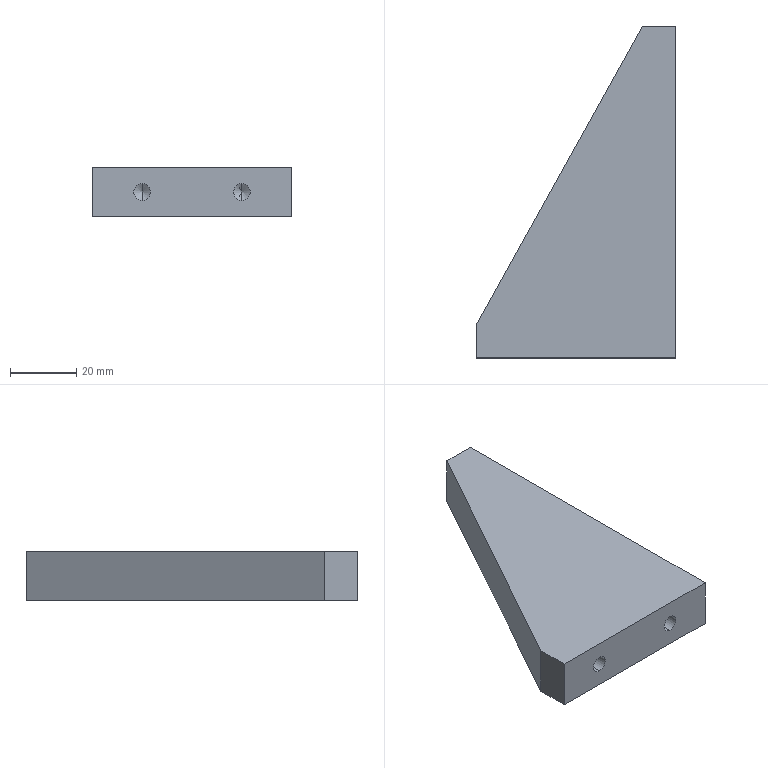Part | SolidWorks | features BaseBody 1 | 1 solid | 27 faces | box 60 x 100 x 15 mm | volume 54728 mm3 | cylinder 10 | cone 10 | plane 7 | commonest cylinder face diameters 5 x10
STEP:
#1=CARTESIAN_POINT('',(-15.,25.,2.5));
#2=VERTEX_POINT('',#1);
#3=CARTESIAN_POINT('',(-15.,25.,-2.5));
#4=VERTEX_POINT('',#3);
#5=CARTESIAN_POINT('',(-15.,25.,0.));
#6=DIRECTION('',(1.,0.,0.));
#7=DIRECTION('',(0.,0.,-1.));
#8=AXIS2_PLACEMENT_3D('',#5,#6,#7);
#9=CIRCLE('',#8,2.5);
#10=EDGE_CURVE('',#2,#4,#9,.T.);
#11=ORIENTED_EDGE('',*,*,#10,.F.);
#12=CARTESIAN_POINT('',(0.,25.,2.5));
#13=VERTEX_POINT('',#12);
#14=CARTESIAN_POINT('',(0.,25.,2.5));
#15=DIRECTION('',(1.,0.,0.));
#16=VECTOR('',#15,1000.);
#17=LINE('',#14,#16);
#18=EDGE_CURVE('',#2,#13,#17,.T.);
#19=ORIENTED_EDGE('',*,*,#18,.T.);
#20=CARTESIAN_POINT('',(0.,25.,-2.5));
#21=VERTEX_POINT('',#20);
#22=CARTESIAN_POINT('',(0.,25.,0.));
#23=DIRECTION('',(1.,0.,0.));
#24=DIRECTION('',(0.,0.,-1.));
#25=AXIS2_PLACEMENT_3D('',#22,#23,#24);
#26=CIRCLE('',#25,2.5);
#27=EDGE_CURVE('',#13,#21,#26,.T.);
#28=ORIENTED_EDGE('',*,*,#27,.T.);
#29=CARTESIAN_POINT('',(0.,25.,-2.5));
#30=DIRECTION('',(1.,0.,0.));
#31=VECTOR('',#30,1000.);
#32=LINE('',#29,#31);
#33=EDGE_CURVE('',#4,#21,#32,.T.);
#34=ORIENTED_EDGE('',*,*,#33,.F.);
#35=EDGE_LOOP('',(#11,#19,#28,#34));
#36=FACE_OUTER_BOUND('',#35,.T.);
#37=CARTESIAN_POINT('',(0.,25.,0.));
#38=DIRECTION('',(1.,0.,0.));
#39=DIRECTION('',(0.,0.,-1.));
#40=AXIS2_PLACEMENT_3D('',#37,#38,#39);
#41=CYLINDRICAL_SURFACE('',#40,2.5);
#42=ADVANCED_FACE('',(#36),#41,.F.);
#43=CARTESIAN_POINT('',(-16.502,25.,0.));
#44=VERTEX_POINT('',#43);
#45=CARTESIAN_POINT('',(-15.,25.,-2.5));
#46=DIRECTION('',(0.515,0.,-0.8572));
#47=VECTOR('',#46,1000.);
#48=LINE('',#45,#47);
#49=EDGE_CURVE('',#44,#4,#48,.T.);
#50=ORIENTED_EDGE('',*,*,#49,.F.);
#51=CARTESIAN_POINT('',(-15.,25.,2.5));
#52=DIRECTION('',(0.515,0.,0.8572));
#53=VECTOR('',#52,1000.);
#54=LINE('',#51,#53);
#55=EDGE_CURVE('',#44,#2,#54,.T.);
#56=ORIENTED_EDGE('',*,*,#55,.T.);
#57=ORIENTED_EDGE('',*,*,#10,.T.);
#58=EDGE_LOOP('',(#50,#56,#57));
#59=FACE_OUTER_BOUND('',#58,.T.);
#60=CARTESIAN_POINT('',(-15.,25.,0.));
#61=DIRECTION('',(1.,0.,0.));
#62=DIRECTION('',(0.,0.,-1.));
#63=AXIS2_PLACEMENT_3D('',#60,#61,#62);
#64=CONICAL_SURFACE('',#63,2.5,1.03);
#65=ADVANCED_FACE('',(#59),#64,.F.);
#66=CARTESIAN_POINT('',(-15.,55.,2.5));
#67=VERTEX_POINT('',#66);
#68=CARTESIAN_POINT('',(-15.,55.,-2.5));
#69=VERTEX_POINT('',#68);
#70=CARTESIAN_POINT('',(-15.,55.,0.));
#71=DIRECTION('',(1.,0.,0.));
#72=DIRECTION('',(0.,0.,-1.));
#73=AXIS2_PLACEMENT_3D('',#70,#71,#72);
#74=CIRCLE('',#73,2.5);
#75=EDGE_CURVE('',#67,#69,#74,.T.);
#76=ORIENTED_EDGE('',*,*,#75,.F.);
#77=CARTESIAN_POINT('',(0.,55.,2.5));
#78=VERTEX_POINT('',#77);
#79=CARTESIAN_POINT('',(0.,55.,2.5));
#80=DIRECTION('',(1.,0.,0.));
#81=VECTOR('',#80,1000.);
#82=LINE('',#79,#81);
#83=EDGE_CURVE('',#67,#78,#82,.T.);
#84=ORIENTED_EDGE('',*,*,#83,.T.);
#85=CARTESIAN_POINT('',(0.,55.,-2.5));
#86=VERTEX_POINT('',#85);
#87=CARTESIAN_POINT('',(0.,55.,0.));
#88=DIRECTION('',(1.,0.,0.));
#89=DIRECTION('',(0.,0.,-1.));
#90=AXIS2_PLACEMENT_3D('',#87,#88,#89);
#91=CIRCLE('',#90,2.5);
#92=EDGE_CURVE('',#78,#86,#91,.T.);
#93=ORIENTED_EDGE('',*,*,#92,.T.);
#94=CARTESIAN_POINT('',(0.,55.,-2.5));
#95=DIRECTION('',(1.,0.,0.));
#96=VECTOR('',#95,1000.);
#97=LINE('',#94,#96);
#98=EDGE_CURVE('',#69,#86,#97,.T.);
#99=ORIENTED_EDGE('',*,*,#98,.F.);
#100=EDGE_LOOP('',(#76,#84,#93,#99));
#101=FACE_OUTER_BOUND('',#100,.T.);
#102=CARTESIAN_POINT('',(0.,55.,0.));
#103=DIRECTION('',(1.,0.,0.));
#104=DIRECTION('',(0.,0.,-1.));
#105=AXIS2_PLACEMENT_3D('',#102,#103,#104);
#106=CYLINDRICAL_SURFACE('',#105,2.5);
#107=ADVANCED_FACE('',(#101),#106,.F.);
#108=CARTESIAN_POINT('',(-16.502,55.,0.));
#109=VERTEX_POINT('',#108);
#110=CARTESIAN_POINT('',(-15.,55.,-2.5));
#111=DIRECTION('',(0.515,0.,-0.8572));
#112=VECTOR('',#111,1000.);
#113=LINE('',#110,#112);
#114=EDGE_CURVE('',#109,#69,#113,.T.);
#115=ORIENTED_EDGE('',*,*,#114,.F.);
#116=CARTESIAN_POINT('',(-15.,55.,2.5));
#117=DIRECTION('',(0.515,0.,0.8572));
#118=VECTOR('',#117,1000.);
#119=LINE('',#116,#118);
#120=EDGE_CURVE('',#109,#67,#119,.T.);
#121=ORIENTED_EDGE('',*,*,#120,.T.);
#122=ORIENTED_EDGE('',*,*,#75,.T.);
#123=EDGE_LOOP('',(#115,#121,#122));
#124=FACE_OUTER_BOUND('',#123,.T.);
#125=CARTESIAN_POINT('',(-15.,55.,0.));
#126=DIRECTION('',(1.,0.,0.));
#127=DIRECTION('',(0.,0.,-1.));
#128=AXIS2_PLACEMENT_3D('',#125,#126,#127);
#129=CONICAL_SURFACE('',#128,2.5,1.03);
#130=ADVANCED_FACE('',(#124),#129,.F.);
#131=CARTESIAN_POINT('',(-15.,85.,2.5));
#132=VERTEX_POINT('',#131);
#133=CARTESIAN_POINT('',(-15.,85.,-2.5));
#134=VERTEX_POINT('',#133);
#135=CARTESIAN_POINT('',(-15.,85.,0.));
#136=DIRECTION('',(1.,0.,0.));
#137=DIRECTION('',(0.,0.,-1.));
#138=AXIS2_PLACEMENT_3D('',#135,#136,#137);
#139=CIRCLE('',#138,2.5);
#140=EDGE_CURVE('',#132,#134,#139,.T.);
#141=ORIENTED_EDGE('',*,*,#140,.F.);
#142=CARTESIAN_POINT('',(0.,85.,2.5));
#143=VERTEX_POINT('',#142);
#144=CARTESIAN_POINT('',(0.,85.,2.5));
#145=DIRECTION('',(1.,0.,0.));
#146=VECTOR('',#145,1000.);
#147=LINE('',#144,#146);
#148=EDGE_CURVE('',#132,#143,#147,.T.);
#149=ORIENTED_EDGE('',*,*,#148,.T.);
#150=CARTESIAN_POINT('',(0.,85.,-2.5));
#151=VERTEX_POINT('',#150);
#152=CARTESIAN_POINT('',(0.,85.,0.));
#153=DIRECTION('',(1.,0.,0.));
#154=DIRECTION('',(0.,0.,-1.));
#155=AXIS2_PLACEMENT_3D('',#152,#153,#154);
#156=CIRCLE('',#155,2.5);
#157=EDGE_CURVE('',#143,#151,#156,.T.);
#158=ORIENTED_EDGE('',*,*,#157,.T.);
#159=CARTESIAN_POINT('',(0.,85.,-2.5));
#160=DIRECTION('',(1.,0.,0.));
#161=VECTOR('',#160,1000.);
#162=LINE('',#159,#161);
#163=EDGE_CURVE('',#134,#151,#162,.T.);
#164=ORIENTED_EDGE('',*,*,#163,.F.);
#165=EDGE_LOOP('',(#141,#149,#158,#164));
#166=FACE_OUTER_BOUND('',#165,.T.);
#167=CARTESIAN_POINT('',(0.,85.,0.));
#168=DIRECTION('',(1.,0.,0.));
#169=DIRECTION('',(0.,0.,-1.));
#170=AXIS2_PLACEMENT_3D('',#167,#168,#169);
#171=CYLINDRICAL_SURFACE('',#170,2.5);
#172=ADVANCED_FACE('',(#166),#171,.F.);
#173=CARTESIAN_POINT('',(-16.502,85.,0.));
#174=VERTEX_POINT('',#173);
#175=CARTESIAN_POINT('',(-15.,85.,-2.5));
#176=DIRECTION('',(0.515,0.,-0.8572));
#177=VECTOR('',#176,1000.);
#178=LINE('',#175,#177);
#179=EDGE_CURVE('',#174,#134,#178,.T.);
#180=ORIENTED_EDGE('',*,*,#179,.F.);
#181=CARTESIAN_POINT('',(-15.,85.,2.5));
#182=DIRECTION('',(0.515,0.,0.8572));
#183=VECTOR('',#182,1000.);
#184=LINE('',#181,#183);
#185=EDGE_CURVE('',#174,#132,#184,.T.);
#186=ORIENTED_EDGE('',*,*,#185,.T.);
#187=ORIENTED_EDGE('',*,*,#140,.T.);
#188=EDGE_LOOP('',(#180,#186,#187));
#189=FACE_OUTER_BOUND('',#188,.T.);
#190=CARTESIAN_POINT('',(-15.,85.,0.));
#191=DIRECTION('',(1.,0.,0.));
#192=DIRECTION('',(0.,0.,-1.));
#193=AXIS2_PLACEMENT_3D('',#190,#191,#192);
#194=CONICAL_SURFACE('',#193,2.5,1.03);
#195=ADVANCED_FACE('',(#189),#194,.F.);
#196=CARTESIAN_POINT('',(-15.,15.,2.5));
#197=VERTEX_POINT('',#196);
#198=CARTESIAN_POINT('',(-15.,15.,-2.5));
#199=VERTEX_POINT('',#198);
#200=CARTESIAN_POINT('',(-15.,15.,0.));
#201=DIRECTION('',(0.,-1.,0.));
#202=DIRECTION('',(0.,0.,-1.));
#203=AXIS2_PLACEMENT_3D('',#200,#201,#202);
#204=CIRCLE('',#203,2.5);
#205=EDGE_CURVE('',#197,#199,#204,.T.);
#206=ORIENTED_EDGE('',*,*,#205,.F.);
#207=CARTESIAN_POINT('',(-15.,0.,2.5));
#208=VERTEX_POINT('',#207);
#209=CARTESIAN_POINT('',(-15.,0.,2.5));
#210=DIRECTION('',(0.,-1.,0.));
#211=VECTOR('',#210,1000.);
#212=LINE('',#209,#211);
#213=EDGE_CURVE('',#197,#208,#212,.T.);
#214=ORIENTED_EDGE('',*,*,#213,.T.);
#215=CARTESIAN_POINT('',(-15.,0.,-2.5));
#216=VERTEX_POINT('',#215);
#217=CARTESIAN_POINT('',(-15.,0.,0.));
#218=DIRECTION('',(0.,-1.,0.));
#219=DIRECTION('',(0.,0.,-1.));
#220=AXIS2_PLACEMENT_3D('',#217,#218,#219);
#221=CIRCLE('',#220,2.5);
#222=EDGE_CURVE('',#208,#216,#221,.T.);
#223=ORIENTED_EDGE('',*,*,#222,.T.);
#224=CARTESIAN_POINT('',(-15.,0.,-2.5));
#225=DIRECTION('',(0.,-1.,0.));
#226=VECTOR('',#225,1000.);
#227=LINE('',#224,#226);
#228=EDGE_CURVE('',#199,#216,#227,.T.);
#229=ORIENTED_EDGE('',*,*,#228,.F.);
#230=EDGE_LOOP('',(#206,#214,#223,#229));
#231=FACE_OUTER_BOUND('',#230,.T.);
#232=CARTESIAN_POINT('',(-15.,0.,0.));
#233=DIRECTION('',(0.,-1.,0.));
#234=DIRECTION('',(0.,0.,-1.));
#235=AXIS2_PLACEMENT_3D('',#232,#233,#234);
#236=CYLINDRICAL_SURFACE('',#235,2.5);
#237=ADVANCED_FACE('',(#231),#236,.F.);
#238=CARTESIAN_POINT('',(-15.,16.502,0.));
#239=VERTEX_POINT('',#238);
#240=CARTESIAN_POINT('',(-15.,15.,-2.5));
#241=DIRECTION('',(0.,-0.515,-0.8572));
#242=VECTOR('',#241,1000.);
#243=LINE('',#240,#242);
#244=EDGE_CURVE('',#239,#199,#243,.T.);
#245=ORIENTED_EDGE('',*,*,#244,.F.);
#246=CARTESIAN_POINT('',(-15.,15.,2.5));
#247=DIRECTION('',(0.,-0.515,0.8572));
#248=VECTOR('',#247,1000.);
#249=LINE('',#246,#248);
#250=EDGE_CURVE('',#239,#197,#249,.T.);
#251=ORIENTED_EDGE('',*,*,#250,.T.);
#252=ORIENTED_EDGE('',*,*,#205,.T.);
#253=EDGE_LOOP('',(#245,#251,#252));
#254=FACE_OUTER_BOUND('',#253,.T.);
#255=CARTESIAN_POINT('',(-15.,15.,0.));
#256=DIRECTION('',(0.,-1.,0.));
#257=DIRECTION('',(0.,0.,-1.));
#258=AXIS2_PLACEMENT_3D('',#255,#256,#257);
#259=CONICAL_SURFACE('',#258,2.5,1.03);
#260=ADVANCED_FACE('',(#254),#259,.F.);
#261=CARTESIAN_POINT('',(-45.,15.,2.5));
#262=VERTEX_POINT('',#261);
#263=CARTESIAN_POINT('',(-45.,15.,-2.5));
#264=VERTEX_POINT('',#263);
#265=CARTESIAN_POINT('',(-45.,15.,0.));
#266=DIRECTION('',(0.,-1.,0.));
#267=DIRECTION('',(0.,0.,-1.));
#268=AXIS2_PLACEMENT_3D('',#265,#266,#267);
#269=CIRCLE('',#268,2.5);
#270=EDGE_CURVE('',#262,#264,#269,.T.);
#271=ORIENTED_EDGE('',*,*,#270,.F.);
#272=CARTESIAN_POINT('',(-45.,0.,2.5));
#273=VERTEX_POINT('',#272);
#274=CARTESIAN_POINT('',(-45.,0.,2.5));
#275=DIRECTION('',(0.,-1.,0.));
#276=VECTOR('',#275,1000.);
#277=LINE('',#274,#276);
#278=EDGE_CURVE('',#262,#273,#277,.T.);
#279=ORIENTED_EDGE('',*,*,#278,.T.);
#280=CARTESIAN_POINT('',(-45.,0.,-2.5));
#281=VERTEX_POINT('',#280);
#282=CARTESIAN_POINT('',(-45.,0.,0.));
#283=DIRECTION('',(0.,-1.,0.));
#284=DIRECTION('',(0.,0.,-1.));
#285=AXIS2_PLACEMENT_3D('',#282,#283,#284);
#286=CIRCLE('',#285,2.5);
#287=EDGE_CURVE('',#273,#281,#286,.T.);
#288=ORIENTED_EDGE('',*,*,#287,.T.);
#289=CARTESIAN_POINT('',(-45.,0.,-2.5));
#290=DIRECTION('',(0.,-1.,0.));
#291=VECTOR('',#290,1000.);
#292=LINE('',#289,#291);
#293=EDGE_CURVE('',#264,#281,#292,.T.);
#294=ORIENTED_EDGE('',*,*,#293,.F.);
#295=EDGE_LOOP('',(#271,#279,#288,#294));
#296=FACE_OUTER_BOUND('',#295,.T.);
#297=CARTESIAN_POINT('',(-45.,0.,0.));
#298=DIRECTION('',(0.,-1.,0.));
#299=DIRECTION('',(0.,0.,-1.));
#300=AXIS2_PLACEMENT_3D('',#297,#298,#299);
#301=CYLINDRICAL_SURFACE('',#300,2.5);
#302=ADVANCED_FACE('',(#296),#301,.F.);
#303=CARTESIAN_POINT('',(-45.,16.502,0.));
#304=VERTEX_POINT('',#303);
#305=CARTESIAN_POINT('',(-45.,15.,-2.5));
#306=DIRECTION('',(0.,-0.515,-0.8572));
#307=VECTOR('',#306,1000.);
#308=LINE('',#305,#307);
#309=EDGE_CURVE('',#304,#264,#308,.T.);
#310=ORIENTED_EDGE('',*,*,#309,.F.);
#311=CARTESIAN_POINT('',(-45.,15.,2.5));
#312=DIRECTION('',(0.,-0.515,0.8572));
#313=VECTOR('',#312,1000.);
#314=LINE('',#311,#313);
#315=EDGE_CURVE('',#304,#262,#314,.T.);
#316=ORIENTED_EDGE('',*,*,#315,.T.);
#317=ORIENTED_EDGE('',*,*,#270,.T.);
#318=EDGE_LOOP('',(#310,#316,#317));
#319=FACE_OUTER_BOUND('',#318,.T.);
#320=CARTESIAN_POINT('',(-45.,15.,0.));
#321=DIRECTION('',(0.,-1.,0.));
#322=DIRECTION('',(0.,0.,-1.));
#323=AXIS2_PLACEMENT_3D('',#320,#321,#322);
#324=CONICAL_SURFACE('',#323,2.5,1.03);
#325=ADVANCED_FACE('',(#319),#324,.F.);
#326=CARTESIAN_POINT('',(-60.,10.,-7.5));
#327=VERTEX_POINT('',#326);
#328=CARTESIAN_POINT('',(-60.,0.,-7.5));
#329=VERTEX_POINT('',#328);
#330=CARTESIAN_POINT('',(-60.,10.,-7.5));
#331=DIRECTION('',(0.,-1.,0.));
#332=VECTOR('',#331,1000.);
#333=LINE('',#330,#332);
#334=EDGE_CURVE('',#327,#329,#333,.T.);
#335=ORIENTED_EDGE('',*,*,#334,.F.);
#336=CARTESIAN_POINT('',(-10.,100.,-7.5));
#337=VERTEX_POINT('',#336);
#338=CARTESIAN_POINT('',(-10.,100.,-7.5));
#339=DIRECTION('',(-0.4856,-0.8742,0.));
#340=VECTOR('',#339,1000.);
#341=LINE('',#338,#340);
#342=EDGE_CURVE('',#337,#327,#341,.T.);
#343=ORIENTED_EDGE('',*,*,#342,.F.);
#344=CARTESIAN_POINT('',(0.,100.,-7.5));
#345=VERTEX_POINT('',#344);
#346=CARTESIAN_POINT('',(0.,100.,-7.5));
#347=DIRECTION('',(-1.,0.,0.));
#348=VECTOR('',#347,1000.);
#349=LINE('',#346,#348);
#350=EDGE_CURVE('',#345,#337,#349,.T.);
#351=ORIENTED_EDGE('',*,*,#350,.F.);
#352=CARTESIAN_POINT('',(0.,0.,-7.5));
#353=VERTEX_POINT('',#352);
#354=CARTESIAN_POINT('',(0.,0.,-7.5));
#355=DIRECTION('',(0.,1.,0.));
#356=VECTOR('',#355,1000.);
#357=LINE('',#354,#356);
#358=EDGE_CURVE('',#353,#345,#357,.T.);
#359=ORIENTED_EDGE('',*,*,#358,.F.);
#360=CARTESIAN_POINT('',(-60.,0.,-7.5));
#361=DIRECTION('',(1.,0.,0.));
#362=VECTOR('',#361,1000.);
#363=LINE('',#360,#362);
#364=EDGE_CURVE('',#329,#353,#363,.T.);
#365=ORIENTED_EDGE('',*,*,#364,.F.);
#366=EDGE_LOOP('',(#335,#343,#351,#359,#365));
#367=FACE_OUTER_BOUND('',#366,.T.);
#368=CARTESIAN_POINT('',(0.,0.,-7.5));
#369=DIRECTION('',(0.,0.,1.));
#370=DIRECTION('',(1.,0.,0.));
#371=AXIS2_PLACEMENT_3D('',#368,#369,#370);
#372=PLANE('',#371);
#373=ADVANCED_FACE('',(#367),#372,.F.);
#374=CARTESIAN_POINT('',(-60.,10.,7.5));
#375=VERTEX_POINT('',#374);
#376=CARTESIAN_POINT('',(-60.,0.,7.5));
#377=VERTEX_POINT('',#376);
#378=CARTESIAN_POINT('',(-60.,10.,7.5));
#379=DIRECTION('',(0.,-1.,0.));
#380=VECTOR('',#379,1000.);
#381=LINE('',#378,#380);
#382=EDGE_CURVE('',#375,#377,#381,.T.);
#383=ORIENTED_EDGE('',*,*,#382,.T.);
#384=CARTESIAN_POINT('',(0.,0.,7.5));
#385=VERTEX_POINT('',#384);
#386=CARTESIAN_POINT('',(-60.,0.,7.5));
#387=DIRECTION('',(1.,0.,0.));
#388=VECTOR('',#387,1000.);
#389=LINE('',#386,#388);
#390=EDGE_CURVE('',#377,#385,#389,.T.);
#391=ORIENTED_EDGE('',*,*,#390,.T.);
#392=CARTESIAN_POINT('',(0.,100.,7.5));
#393=VERTEX_POINT('',#392);
#394=CARTESIAN_POINT('',(0.,0.,7.5));
#395=DIRECTION('',(0.,1.,0.));
#396=VECTOR('',#395,1000.);
#397=LINE('',#394,#396);
#398=EDGE_CURVE('',#385,#393,#397,.T.);
#399=ORIENTED_EDGE('',*,*,#398,.T.);
#400=CARTESIAN_POINT('',(-10.,100.,7.5));
#401=VERTEX_POINT('',#400);
#402=CARTESIAN_POINT('',(0.,100.,7.5));
#403=DIRECTION('',(-1.,0.,0.));
#404=VECTOR('',#403,1000.);
#405=LINE('',#402,#404);
#406=EDGE_CURVE('',#393,#401,#405,.T.);
#407=ORIENTED_EDGE('',*,*,#406,.T.);
#408=CARTESIAN_POINT('',(-10.,100.,7.5));
#409=DIRECTION('',(-0.4856,-0.8742,0.));
#410=VECTOR('',#409,1000.);
#411=LINE('',#408,#410);
#412=EDGE_CURVE('',#401,#375,#411,.T.);
#413=ORIENTED_EDGE('',*,*,#412,.T.);
#414=EDGE_LOOP('',(#383,#391,#399,#407,#413));
#415=FACE_OUTER_BOUND('',#414,.T.);
#416=CARTESIAN_POINT('',(0.,0.,7.5));
#417=DIRECTION('',(0.,0.,1.));
#418=DIRECTION('',(1.,0.,0.));
#419=AXIS2_PLACEMENT_3D('',#416,#417,#418);
#420=PLANE('',#419);
#421=ADVANCED_FACE('',(#415),#420,.T.);
#422=ORIENTED_EDGE('',*,*,#342,.T.);
#423=CARTESIAN_POINT('',(-60.,10.,7.5));
#424=DIRECTION('',(0.,0.,-1.));
#425=VECTOR('',#424,1000.);
#426=LINE('',#423,#425);
#427=EDGE_CURVE('',#375,#327,#426,.T.);
#428=ORIENTED_EDGE('',*,*,#427,.F.);
#429=ORIENTED_EDGE('',*,*,#412,.F.);
#430=CARTESIAN_POINT('',(-10.,100.,7.5));
#431=DIRECTION('',(0.,0.,-1.));
#432=VECTOR('',#431,1000.);
#433=LINE('',#430,#432);
#434=EDGE_CURVE('',#401,#337,#433,.T.);
#435=ORIENTED_EDGE('',*,*,#434,.T.);
#436=EDGE_LOOP('',(#422,#428,#429,#435));
#437=FACE_OUTER_BOUND('',#436,.T.);
#438=CARTESIAN_POINT('',(-10.,100.,7.5));
#439=DIRECTION('',(0.8742,-0.4856,0.));
#440=DIRECTION('',(0.,0.,-1.));
#441=AXIS2_PLACEMENT_3D('',#438,#439,#440);
#442=PLANE('',#441);
#443=ADVANCED_FACE('',(#437),#442,.F.);
#444=ORIENTED_EDGE('',*,*,#350,.T.);
#445=ORIENTED_EDGE('',*,*,#434,.F.);
#446=ORIENTED_EDGE('',*,*,#406,.F.);
#447=CARTESIAN_POINT('',(0.,100.,7.5));
#448=DIRECTION('',(0.,0.,-1.));
#449=VECTOR('',#448,1000.);
#450=LINE('',#447,#449);
#451=EDGE_CURVE('',#393,#345,#450,.T.);
#452=ORIENTED_EDGE('',*,*,#451,.T.);
#453=EDGE_LOOP('',(#444,#445,#446,#452));
#454=FACE_OUTER_BOUND('',#453,.T.);
#455=CARTESIAN_POINT('',(0.,100.,7.5));
#456=DIRECTION('',(0.,-1.,0.));
#457=DIRECTION('',(0.,0.,-1.));
#458=AXIS2_PLACEMENT_3D('',#455,#456,#457);
#459=PLANE('',#458);
#460=ADVANCED_FACE('',(#454),#459,.F.);
#461=CARTESIAN_POINT('',(0.,85.,0.));
#462=DIRECTION('',(1.,0.,0.));
#463=DIRECTION('',(0.,0.,-1.));
#464=AXIS2_PLACEMENT_3D('',#461,#462,#463);
#465=CIRCLE('',#464,2.5);
#466=EDGE_CURVE('',#151,#143,#465,.T.);
#467=ORIENTED_EDGE('',*,*,#466,.F.);
#468=ORIENTED_EDGE('',*,*,#157,.F.);
#469=EDGE_LOOP('',(#467,#468));
#470=FACE_BOUND('',#469,.T.);
#471=CARTESIAN_POINT('',(0.,55.,0.));
#472=DIRECTION('',(1.,0.,0.));
#473=DIRECTION('',(0.,0.,-1.));
#474=AXIS2_PLACEMENT_3D('',#471,#472,#473);
#475=CIRCLE('',#474,2.5);
#476=EDGE_CURVE('',#86,#78,#475,.T.);
#477=ORIENTED_EDGE('',*,*,#476,.F.);
#478=ORIENTED_EDGE('',*,*,#92,.F.);
#479=EDGE_LOOP('',(#477,#478));
#480=FACE_BOUND('',#479,.T.);
#481=CARTESIAN_POINT('',(0.,25.,0.));
#482=DIRECTION('',(1.,0.,0.));
#483=DIRECTION('',(0.,0.,-1.));
#484=AXIS2_PLACEMENT_3D('',#481,#482,#483);
#485=CIRCLE('',#484,2.5);
#486=EDGE_CURVE('',#21,#13,#485,.T.);
#487=ORIENTED_EDGE('',*,*,#486,.F.);
#488=ORIENTED_EDGE('',*,*,#27,.F.);
#489=EDGE_LOOP('',(#487,#488));
#490=FACE_BOUND('',#489,.T.);
#491=ORIENTED_EDGE('',*,*,#358,.T.);
#492=ORIENTED_EDGE('',*,*,#451,.F.);
#493=ORIENTED_EDGE('',*,*,#398,.F.);
#494=CARTESIAN_POINT('',(0.,0.,7.5));
#495=DIRECTION('',(0.,0.,-1.));
#496=VECTOR('',#495,1000.);
#497=LINE('',#494,#496);
#498=EDGE_CURVE('',#385,#353,#497,.T.);
#499=ORIENTED_EDGE('',*,*,#498,.T.);
#500=EDGE_LOOP('',(#491,#492,#493,#499));
#501=FACE_OUTER_BOUND('',#500,.T.);
#502=CARTESIAN_POINT('',(0.,0.,7.5));
#503=DIRECTION('',(-1.,0.,0.));
#504=DIRECTION('',(0.,0.,1.));
#505=AXIS2_PLACEMENT_3D('',#502,#503,#504);
#506=PLANE('',#505);
#507=ADVANCED_FACE('',(#470,#480,#490,#501),#506,.F.);
#508=CARTESIAN_POINT('',(-45.,0.,0.));
#509=DIRECTION('',(0.,-1.,0.));
#510=DIRECTION('',(0.,0.,-1.));
#511=AXIS2_PLACEMENT_3D('',#508,#509,#510);
#512=CIRCLE('',#511,2.5);
#513=EDGE_CURVE('',#281,#273,#512,.T.);
#514=ORIENTED_EDGE('',*,*,#513,.F.);
#515=ORIENTED_EDGE('',*,*,#287,.F.);
#516=EDGE_LOOP('',(#514,#515));
#517=FACE_BOUND('',#516,.T.);
#518=CARTESIAN_POINT('',(-15.,0.,0.));
#519=DIRECTION('',(0.,-1.,0.));
#520=DIRECTION('',(0.,0.,-1.));
#521=AXIS2_PLACEMENT_3D('',#518,#519,#520);
#522=CIRCLE('',#521,2.5);
#523=EDGE_CURVE('',#216,#208,#522,.T.);
#524=ORIENTED_EDGE('',*,*,#523,.F.);
#525=ORIENTED_EDGE('',*,*,#222,.F.);
#526=EDGE_LOOP('',(#524,#525));
#527=FACE_BOUND('',#526,.T.);
#528=ORIENTED_EDGE('',*,*,#364,.T.);
#529=ORIENTED_EDGE('',*,*,#498,.F.);
#530=ORIENTED_EDGE('',*,*,#390,.F.);
#531=CARTESIAN_POINT('',(-60.,0.,7.5));
#532=DIRECTION('',(0.,0.,-1.));
#533=VECTOR('',#532,1000.);
#534=LINE('',#531,#533);
#535=EDGE_CURVE('',#377,#329,#534,.T.);
#536=ORIENTED_EDGE('',*,*,#535,.T.);
#537=EDGE_LOOP('',(#528,#529,#530,#536));
#538=FACE_OUTER_BOUND('',#537,.T.);
#539=CARTESIAN_POINT('',(-60.,0.,7.5));
#540=DIRECTION('',(0.,1.,0.));
#541=DIRECTION('',(1.,0.,0.));
#542=AXIS2_PLACEMENT_3D('',#539,#540,#541);
#543=PLANE('',#542);
#544=ADVANCED_FACE('',(#517,#527,#538),#543,.F.);
#545=ORIENTED_EDGE('',*,*,#334,.T.);
#546=ORIENTED_EDGE('',*,*,#535,.F.);
#547=ORIENTED_EDGE('',*,*,#382,.F.);
#548=ORIENTED_EDGE('',*,*,#427,.T.);
#549=EDGE_LOOP('',(#545,#546,#547,#548));
#550=FACE_OUTER_BOUND('',#549,.T.);
#551=CARTESIAN_POINT('',(-60.,10.,7.5));
#552=DIRECTION('',(1.,0.,0.));
#553=DIRECTION('',(0.,1.,0.));
#554=AXIS2_PLACEMENT_3D('',#551,#552,#553);
#555=PLANE('',#554);
#556=ADVANCED_FACE('',(#550),#555,.F.);
#557=ORIENTED_EDGE('',*,*,#315,.F.);
#558=ORIENTED_EDGE('',*,*,#309,.T.);
#559=CARTESIAN_POINT('',(-45.,15.,0.));
#560=DIRECTION('',(0.,-1.,0.));
#561=DIRECTION('',(0.,0.,-1.));
#562=AXIS2_PLACEMENT_3D('',#559,#560,#561);
#563=CIRCLE('',#562,2.5);
#564=EDGE_CURVE('',#264,#262,#563,.T.);
#565=ORIENTED_EDGE('',*,*,#564,.T.);
#566=EDGE_LOOP('',(#557,#558,#565));
#567=FACE_OUTER_BOUND('',#566,.T.);
#568=CARTESIAN_POINT('',(-45.,15.,0.));
#569=DIRECTION('',(0.,-1.,0.));
#570=DIRECTION('',(0.,0.,-1.));
#571=AXIS2_PLACEMENT_3D('',#568,#569,#570);
#572=CONICAL_SURFACE('',#571,2.5,1.03);
#573=ADVANCED_FACE('',(#567),#572,.F.);
#574=ORIENTED_EDGE('',*,*,#278,.F.);
#575=ORIENTED_EDGE('',*,*,#564,.F.);
#576=ORIENTED_EDGE('',*,*,#293,.T.);
#577=ORIENTED_EDGE('',*,*,#513,.T.);
#578=EDGE_LOOP('',(#574,#575,#576,#577));
#579=FACE_OUTER_BOUND('',#578,.T.);
#580=CARTESIAN_POINT('',(-45.,0.,0.));
#581=DIRECTION('',(0.,-1.,0.));
#582=DIRECTION('',(0.,0.,-1.));
#583=AXIS2_PLACEMENT_3D('',#580,#581,#582);
#584=CYLINDRICAL_SURFACE('',#583,2.5);
#585=ADVANCED_FACE('',(#579),#584,.F.);
#586=ORIENTED_EDGE('',*,*,#250,.F.);
#587=ORIENTED_EDGE('',*,*,#244,.T.);
#588=CARTESIAN_POINT('',(-15.,15.,0.));
#589=DIRECTION('',(0.,-1.,0.));
#590=DIRECTION('',(0.,0.,-1.));
#591=AXIS2_PLACEMENT_3D('',#588,#589,#590);
#592=CIRCLE('',#591,2.5);
#593=EDGE_CURVE('',#199,#197,#592,.T.);
#594=ORIENTED_EDGE('',*,*,#593,.T.);
#595=EDGE_LOOP('',(#586,#587,#594));
#596=FACE_OUTER_BOUND('',#595,.T.);
#597=CARTESIAN_POINT('',(-15.,15.,0.));
#598=DIRECTION('',(0.,-1.,0.));
#599=DIRECTION('',(0.,0.,-1.));
#600=AXIS2_PLACEMENT_3D('',#597,#598,#599);
#601=CONICAL_SURFACE('',#600,2.5,1.03);
#602=ADVANCED_FACE('',(#596),#601,.F.);
#603=ORIENTED_EDGE('',*,*,#213,.F.);
#604=ORIENTED_EDGE('',*,*,#593,.F.);
#605=ORIENTED_EDGE('',*,*,#228,.T.);
#606=ORIENTED_EDGE('',*,*,#523,.T.);
#607=EDGE_LOOP('',(#603,#604,#605,#606));
#608=FACE_OUTER_BOUND('',#607,.T.);
#609=CARTESIAN_POINT('',(-15.,0.,0.));
#610=DIRECTION('',(0.,-1.,0.));
#611=DIRECTION('',(0.,0.,-1.));
#612=AXIS2_PLACEMENT_3D('',#609,#610,#611);
#613=CYLINDRICAL_SURFACE('',#612,2.5);
#614=ADVANCED_FACE('',(#608),#613,.F.);
#615=ORIENTED_EDGE('',*,*,#185,.F.);
#616=ORIENTED_EDGE('',*,*,#179,.T.);
#617=CARTESIAN_POINT('',(-15.,85.,0.));
#618=DIRECTION('',(1.,0.,0.));
#619=DIRECTION('',(0.,0.,-1.));
#620=AXIS2_PLACEMENT_3D('',#617,#618,#619);
#621=CIRCLE('',#620,2.5);
#622=EDGE_CURVE('',#134,#132,#621,.T.);
#623=ORIENTED_EDGE('',*,*,#622,.T.);
#624=EDGE_LOOP('',(#615,#616,#623));
#625=FACE_OUTER_BOUND('',#624,.T.);
#626=CARTESIAN_POINT('',(-15.,85.,0.));
#627=DIRECTION('',(1.,0.,0.));
#628=DIRECTION('',(0.,0.,-1.));
#629=AXIS2_PLACEMENT_3D('',#626,#627,#628);
#630=CONICAL_SURFACE('',#629,2.5,1.03);
#631=ADVANCED_FACE('',(#625),#630,.F.);
#632=ORIENTED_EDGE('',*,*,#148,.F.);
#633=ORIENTED_EDGE('',*,*,#622,.F.);
#634=ORIENTED_EDGE('',*,*,#163,.T.);
#635=ORIENTED_EDGE('',*,*,#466,.T.);
#636=EDGE_LOOP('',(#632,#633,#634,#635));
#637=FACE_OUTER_BOUND('',#636,.T.);
#638=CARTESIAN_POINT('',(0.,85.,0.));
#639=DIRECTION('',(1.,0.,0.));
#640=DIRECTION('',(0.,0.,-1.));
#641=AXIS2_PLACEMENT_3D('',#638,#639,#640);
#642=CYLINDRICAL_SURFACE('',#641,2.5);
#643=ADVANCED_FACE('',(#637),#642,.F.);
#644=ORIENTED_EDGE('',*,*,#120,.F.);
#645=ORIENTED_EDGE('',*,*,#114,.T.);
#646=CARTESIAN_POINT('',(-15.,55.,0.));
#647=DIRECTION('',(1.,0.,0.));
#648=DIRECTION('',(0.,0.,-1.));
#649=AXIS2_PLACEMENT_3D('',#646,#647,#648);
#650=CIRCLE('',#649,2.5);
#651=EDGE_CURVE('',#69,#67,#650,.T.);
#652=ORIENTED_EDGE('',*,*,#651,.T.);
#653=EDGE_LOOP('',(#644,#645,#652));
#654=FACE_OUTER_BOUND('',#653,.T.);
#655=CARTESIAN_POINT('',(-15.,55.,0.));
#656=DIRECTION('',(1.,0.,0.));
#657=DIRECTION('',(0.,0.,-1.));
#658=AXIS2_PLACEMENT_3D('',#655,#656,#657);
#659=CONICAL_SURFACE('',#658,2.5,1.03);
#660=ADVANCED_FACE('',(#654),#659,.F.);
#661=ORIENTED_EDGE('',*,*,#83,.F.);
#662=ORIENTED_EDGE('',*,*,#651,.F.);
#663=ORIENTED_EDGE('',*,*,#98,.T.);
#664=ORIENTED_EDGE('',*,*,#476,.T.);
#665=EDGE_LOOP('',(#661,#662,#663,#664));
#666=FACE_OUTER_BOUND('',#665,.T.);
#667=CARTESIAN_POINT('',(0.,55.,0.));
#668=DIRECTION('',(1.,0.,0.));
#669=DIRECTION('',(0.,0.,-1.));
#670=AXIS2_PLACEMENT_3D('',#667,#668,#669);
#671=CYLINDRICAL_SURFACE('',#670,2.5);
#672=ADVANCED_FACE('',(#666),#671,.F.);
#673=ORIENTED_EDGE('',*,*,#55,.F.);
#674=ORIENTED_EDGE('',*,*,#49,.T.);
#675=CARTESIAN_POINT('',(-15.,25.,0.));
#676=DIRECTION('',(1.,0.,0.));
#677=DIRECTION('',(0.,0.,-1.));
#678=AXIS2_PLACEMENT_3D('',#675,#676,#677);
#679=CIRCLE('',#678,2.5);
#680=EDGE_CURVE('',#4,#2,#679,.T.);
#681=ORIENTED_EDGE('',*,*,#680,.T.);
#682=EDGE_LOOP('',(#673,#674,#681));
#683=FACE_OUTER_BOUND('',#682,.T.);
#684=CARTESIAN_POINT('',(-15.,25.,0.));
#685=DIRECTION('',(1.,0.,0.));
#686=DIRECTION('',(0.,0.,-1.));
#687=AXIS2_PLACEMENT_3D('',#684,#685,#686);
#688=CONICAL_SURFACE('',#687,2.5,1.03);
#689=ADVANCED_FACE('',(#683),#688,.F.);
#690=ORIENTED_EDGE('',*,*,#18,.F.);
#691=ORIENTED_EDGE('',*,*,#680,.F.);
#692=ORIENTED_EDGE('',*,*,#33,.T.);
#693=ORIENTED_EDGE('',*,*,#486,.T.);
#694=EDGE_LOOP('',(#690,#691,#692,#693));
#695=FACE_OUTER_BOUND('',#694,.T.);
#696=CARTESIAN_POINT('',(0.,25.,0.));
#697=DIRECTION('',(1.,0.,0.));
#698=DIRECTION('',(0.,0.,-1.));
#699=AXIS2_PLACEMENT_3D('',#696,#697,#698);
#700=CYLINDRICAL_SURFACE('',#699,2.5);
#701=ADVANCED_FACE('',(#695),#700,.F.);
#702=CLOSED_SHELL('',(#42,#65,#107,#130,#172,#195,#237,#260,#302,#325,#373,#421,#443,#460,#507,#544,#556,#573,#585,#602,#614,#631,#643,#660,#672,#689,#701));
#703=MANIFOLD_SOLID_BREP('',#702);
#704=CARTESIAN_POINT('',(0.,0.,0.));
#705=DIRECTION('',(0.,0.,1.));
#706=DIRECTION('',(1.,0.,0.));
#707=AXIS2_PLACEMENT_3D('',#704,#705,#706);
#708=(LENGTH_UNIT()NAMED_UNIT(*)SI_UNIT(.MILLI.,.METRE.));
#709=UNCERTAINTY_MEASURE_WITH_UNIT(LENGTH_MEASURE(0.00001),#708,'','');
#710=(NAMED_UNIT(*)PLANE_ANGLE_UNIT()SI_UNIT($,.RADIAN.));
#711=(NAMED_UNIT(*)SI_UNIT($,.STERADIAN.)SOLID_ANGLE_UNIT());
#712=(GEOMETRIC_REPRESENTATION_CONTEXT(3)GLOBAL_UNCERTAINTY_ASSIGNED_CONTEXT((#709))GLOBAL_UNIT_ASSIGNED_CONTEXT((#708,#710,#711))REPRESENTATION_CONTEXT('',''));
#713=ADVANCED_BREP_SHAPE_REPRESENTATION('',(#703,#707),#712);